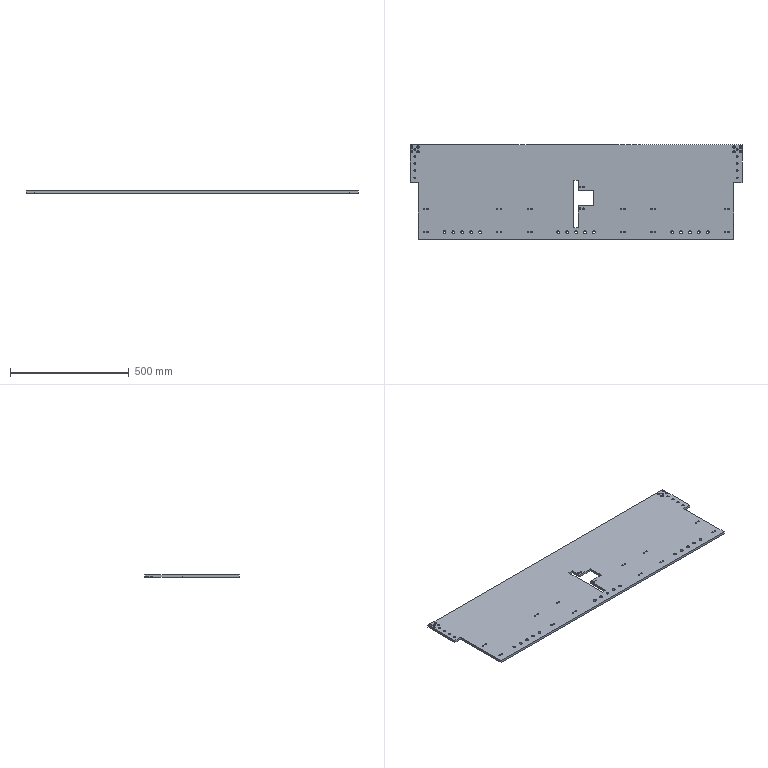Part | NX | features SIMPLE HOLE 43, SYMBOLIC_THREAD 43, CBORE_HOLE 18, DATUM_CSYS 18, EXTRACT_FACE 17, SKETCH 17, HOLE PACKAGE 15, Instance Feature 6, EXTRUDE 2, Mirror Feature 2, Pattern Feature 1 | 1 solid | 201 faces | box 1400 x 400 x 10 mm | volume 5316360 mm3 | cone 86 | cylinder 79 | plane 36 | commonest cylinder face diameters 5.2 x28 6.5 x18 11 x18 10.9 x15